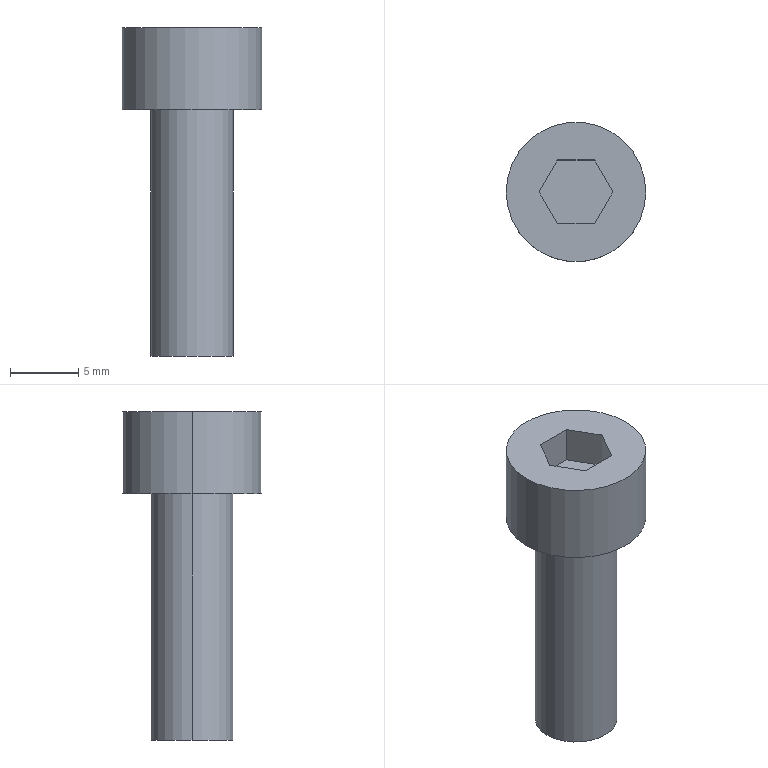Part | SolidWorks | features BaseBody 1 | 1 solid | 14 faces | box 10.2 x 10.2 x 24 mm | volume 948.077 mm3 | plane 10 | cylinder 4 | commonest cylinder face diameters 6 x2 10.2 x2
STEP:
#1=CARTESIAN_POINT('',(3.,0.,-18.));
#2=VERTEX_POINT('',#1);
#3=CARTESIAN_POINT('',(-3.,0.,-18.));
#4=VERTEX_POINT('',#3);
#5=CARTESIAN_POINT('',(0.,0.,-18.));
#6=DIRECTION('',(0.,0.,1.));
#7=DIRECTION('',(1.,0.,0.));
#8=AXIS2_PLACEMENT_3D('',#5,#6,#7);
#9=CIRCLE('',#8,3.);
#10=EDGE_CURVE('',#2,#4,#9,.T.);
#11=ORIENTED_EDGE('',*,*,#10,.T.);
#12=CARTESIAN_POINT('',(-3.,0.,0.));
#13=VERTEX_POINT('',#12);
#14=CARTESIAN_POINT('',(-3.,0.,-18.));
#15=DIRECTION('',(0.,0.,1.));
#16=VECTOR('',#15,1000.);
#17=LINE('',#14,#16);
#18=EDGE_CURVE('',#4,#13,#17,.T.);
#19=ORIENTED_EDGE('',*,*,#18,.T.);
#20=CARTESIAN_POINT('',(3.,0.,0.));
#21=VERTEX_POINT('',#20);
#22=CARTESIAN_POINT('',(0.,0.,0.));
#23=DIRECTION('',(0.,0.,-1.));
#24=DIRECTION('',(1.,0.,0.));
#25=AXIS2_PLACEMENT_3D('',#22,#23,#24);
#26=CIRCLE('',#25,3.);
#27=EDGE_CURVE('',#13,#21,#26,.T.);
#28=ORIENTED_EDGE('',*,*,#27,.T.);
#29=CARTESIAN_POINT('',(3.,0.,-18.));
#30=DIRECTION('',(0.,0.,1.));
#31=VECTOR('',#30,1000.);
#32=LINE('',#29,#31);
#33=EDGE_CURVE('',#2,#21,#32,.T.);
#34=ORIENTED_EDGE('',*,*,#33,.F.);
#35=EDGE_LOOP('',(#11,#19,#28,#34));
#36=FACE_OUTER_BOUND('',#35,.T.);
#37=CARTESIAN_POINT('',(0.,0.,-18.));
#38=DIRECTION('',(0.,0.,1.));
#39=DIRECTION('',(1.,0.,0.));
#40=AXIS2_PLACEMENT_3D('',#37,#38,#39);
#41=CYLINDRICAL_SURFACE('',#40,3.);
#42=ADVANCED_FACE('',(#36),#41,.T.);
#43=CARTESIAN_POINT('',(5.1,0.,0.));
#44=VERTEX_POINT('',#43);
#45=CARTESIAN_POINT('',(-5.1,0.,0.));
#46=VERTEX_POINT('',#45);
#47=CARTESIAN_POINT('',(0.,0.,0.));
#48=DIRECTION('',(0.,0.,1.));
#49=DIRECTION('',(1.,0.,0.));
#50=AXIS2_PLACEMENT_3D('',#47,#48,#49);
#51=CIRCLE('',#50,5.1);
#52=EDGE_CURVE('',#44,#46,#51,.T.);
#53=ORIENTED_EDGE('',*,*,#52,.T.);
#54=CARTESIAN_POINT('',(-5.1,0.,6.));
#55=VERTEX_POINT('',#54);
#56=CARTESIAN_POINT('',(-5.1,0.,0.));
#57=DIRECTION('',(0.,0.,1.));
#58=VECTOR('',#57,1000.);
#59=LINE('',#56,#58);
#60=EDGE_CURVE('',#46,#55,#59,.T.);
#61=ORIENTED_EDGE('',*,*,#60,.T.);
#62=CARTESIAN_POINT('',(5.1,0.,6.));
#63=VERTEX_POINT('',#62);
#64=CARTESIAN_POINT('',(0.,0.,6.));
#65=DIRECTION('',(0.,0.,-1.));
#66=DIRECTION('',(1.,0.,0.));
#67=AXIS2_PLACEMENT_3D('',#64,#65,#66);
#68=CIRCLE('',#67,5.1);
#69=EDGE_CURVE('',#55,#63,#68,.T.);
#70=ORIENTED_EDGE('',*,*,#69,.T.);
#71=CARTESIAN_POINT('',(5.1,0.,0.));
#72=DIRECTION('',(0.,0.,1.));
#73=VECTOR('',#72,1000.);
#74=LINE('',#71,#73);
#75=EDGE_CURVE('',#44,#63,#74,.T.);
#76=ORIENTED_EDGE('',*,*,#75,.F.);
#77=EDGE_LOOP('',(#53,#61,#70,#76));
#78=FACE_OUTER_BOUND('',#77,.T.);
#79=CARTESIAN_POINT('',(0.,0.,0.));
#80=DIRECTION('',(0.,0.,1.));
#81=DIRECTION('',(1.,0.,0.));
#82=AXIS2_PLACEMENT_3D('',#79,#80,#81);
#83=CYLINDRICAL_SURFACE('',#82,5.1);
#84=ADVANCED_FACE('',(#78),#83,.T.);
#85=ORIENTED_EDGE('',*,*,#18,.F.);
#86=CARTESIAN_POINT('',(0.,0.,-18.));
#87=DIRECTION('',(0.,0.,1.));
#88=DIRECTION('',(1.,0.,0.));
#89=AXIS2_PLACEMENT_3D('',#86,#87,#88);
#90=CIRCLE('',#89,3.);
#91=EDGE_CURVE('',#4,#2,#90,.T.);
#92=ORIENTED_EDGE('',*,*,#91,.T.);
#93=ORIENTED_EDGE('',*,*,#33,.T.);
#94=CARTESIAN_POINT('',(0.,0.,0.));
#95=DIRECTION('',(0.,0.,-1.));
#96=DIRECTION('',(1.,0.,0.));
#97=AXIS2_PLACEMENT_3D('',#94,#95,#96);
#98=CIRCLE('',#97,3.);
#99=EDGE_CURVE('',#21,#13,#98,.T.);
#100=ORIENTED_EDGE('',*,*,#99,.T.);
#101=EDGE_LOOP('',(#85,#92,#93,#100));
#102=FACE_OUTER_BOUND('',#101,.T.);
#103=CARTESIAN_POINT('',(0.,0.,-18.));
#104=DIRECTION('',(0.,0.,1.));
#105=DIRECTION('',(1.,0.,0.));
#106=AXIS2_PLACEMENT_3D('',#103,#104,#105);
#107=CYLINDRICAL_SURFACE('',#106,3.);
#108=ADVANCED_FACE('',(#102),#107,.T.);
#109=ORIENTED_EDGE('',*,*,#10,.F.);
#110=ORIENTED_EDGE('',*,*,#91,.F.);
#111=EDGE_LOOP('',(#109,#110));
#112=FACE_OUTER_BOUND('',#111,.T.);
#113=CARTESIAN_POINT('',(0.,0.,-18.));
#114=DIRECTION('',(0.,0.,1.));
#115=DIRECTION('',(1.,0.,0.));
#116=AXIS2_PLACEMENT_3D('',#113,#114,#115);
#117=PLANE('',#116);
#118=ADVANCED_FACE('',(#112),#117,.F.);
#119=ORIENTED_EDGE('',*,*,#99,.F.);
#120=ORIENTED_EDGE('',*,*,#27,.F.);
#121=EDGE_LOOP('',(#119,#120));
#122=FACE_BOUND('',#121,.T.);
#123=ORIENTED_EDGE('',*,*,#52,.F.);
#124=CARTESIAN_POINT('',(0.,0.,0.));
#125=DIRECTION('',(0.,0.,1.));
#126=DIRECTION('',(1.,0.,0.));
#127=AXIS2_PLACEMENT_3D('',#124,#125,#126);
#128=CIRCLE('',#127,5.1);
#129=EDGE_CURVE('',#46,#44,#128,.T.);
#130=ORIENTED_EDGE('',*,*,#129,.F.);
#131=EDGE_LOOP('',(#123,#130));
#132=FACE_OUTER_BOUND('',#131,.T.);
#133=CARTESIAN_POINT('',(0.,0.,0.));
#134=DIRECTION('',(0.,0.,1.));
#135=DIRECTION('',(1.,0.,0.));
#136=AXIS2_PLACEMENT_3D('',#133,#134,#135);
#137=PLANE('',#136);
#138=ADVANCED_FACE('',(#122,#132),#137,.F.);
#139=ORIENTED_EDGE('',*,*,#60,.F.);
#140=ORIENTED_EDGE('',*,*,#129,.T.);
#141=ORIENTED_EDGE('',*,*,#75,.T.);
#142=CARTESIAN_POINT('',(0.,0.,6.));
#143=DIRECTION('',(0.,0.,-1.));
#144=DIRECTION('',(1.,0.,0.));
#145=AXIS2_PLACEMENT_3D('',#142,#143,#144);
#146=CIRCLE('',#145,5.1);
#147=EDGE_CURVE('',#63,#55,#146,.T.);
#148=ORIENTED_EDGE('',*,*,#147,.T.);
#149=EDGE_LOOP('',(#139,#140,#141,#148));
#150=FACE_OUTER_BOUND('',#149,.T.);
#151=CARTESIAN_POINT('',(0.,0.,0.));
#152=DIRECTION('',(0.,0.,1.));
#153=DIRECTION('',(1.,0.,0.));
#154=AXIS2_PLACEMENT_3D('',#151,#152,#153);
#155=CYLINDRICAL_SURFACE('',#154,5.1);
#156=ADVANCED_FACE('',(#150),#155,.T.);
#157=CARTESIAN_POINT('',(-1.35,-2.338,6.));
#158=VERTEX_POINT('',#157);
#159=CARTESIAN_POINT('',(-2.7,0.,6.));
#160=VERTEX_POINT('',#159);
#161=CARTESIAN_POINT('',(-1.35,-2.338,6.));
#162=DIRECTION('',(-0.5,0.866,0.));
#163=VECTOR('',#162,1000.);
#164=LINE('',#161,#163);
#165=EDGE_CURVE('',#158,#160,#164,.T.);
#166=ORIENTED_EDGE('',*,*,#165,.T.);
#167=CARTESIAN_POINT('',(-1.35,2.338,6.));
#168=VERTEX_POINT('',#167);
#169=CARTESIAN_POINT('',(-2.7,0.,6.));
#170=DIRECTION('',(0.5,0.866,0.));
#171=VECTOR('',#170,1000.);
#172=LINE('',#169,#171);
#173=EDGE_CURVE('',#160,#168,#172,.T.);
#174=ORIENTED_EDGE('',*,*,#173,.T.);
#175=CARTESIAN_POINT('',(1.35,2.338,6.));
#176=VERTEX_POINT('',#175);
#177=CARTESIAN_POINT('',(0.,2.338,6.));
#178=DIRECTION('',(1.,0.,0.));
#179=VECTOR('',#178,1000.);
#180=LINE('',#177,#179);
#181=EDGE_CURVE('',#168,#176,#180,.T.);
#182=ORIENTED_EDGE('',*,*,#181,.T.);
#183=CARTESIAN_POINT('',(2.7,0.,6.));
#184=VERTEX_POINT('',#183);
#185=CARTESIAN_POINT('',(1.35,2.338,6.));
#186=DIRECTION('',(0.5,-0.866,0.));
#187=VECTOR('',#186,1000.);
#188=LINE('',#185,#187);
#189=EDGE_CURVE('',#176,#184,#188,.T.);
#190=ORIENTED_EDGE('',*,*,#189,.T.);
#191=CARTESIAN_POINT('',(1.35,-2.338,6.));
#192=VERTEX_POINT('',#191);
#193=CARTESIAN_POINT('',(2.7,0.,6.));
#194=DIRECTION('',(-0.5,-0.866,0.));
#195=VECTOR('',#194,1000.);
#196=LINE('',#193,#195);
#197=EDGE_CURVE('',#184,#192,#196,.T.);
#198=ORIENTED_EDGE('',*,*,#197,.T.);
#199=CARTESIAN_POINT('',(0.,-2.338,6.));
#200=DIRECTION('',(-1.,0.,0.));
#201=VECTOR('',#200,1000.);
#202=LINE('',#199,#201);
#203=EDGE_CURVE('',#192,#158,#202,.T.);
#204=ORIENTED_EDGE('',*,*,#203,.T.);
#205=EDGE_LOOP('',(#166,#174,#182,#190,#198,#204));
#206=FACE_BOUND('',#205,.T.);
#207=ORIENTED_EDGE('',*,*,#147,.F.);
#208=ORIENTED_EDGE('',*,*,#69,.F.);
#209=EDGE_LOOP('',(#207,#208));
#210=FACE_OUTER_BOUND('',#209,.T.);
#211=CARTESIAN_POINT('',(0.,0.,6.));
#212=DIRECTION('',(0.,0.,1.));
#213=DIRECTION('',(1.,0.,0.));
#214=AXIS2_PLACEMENT_3D('',#211,#212,#213);
#215=PLANE('',#214);
#216=ADVANCED_FACE('',(#206,#210),#215,.T.);
#217=ORIENTED_EDGE('',*,*,#173,.F.);
#218=CARTESIAN_POINT('',(-2.7,0.,3.3));
#219=VERTEX_POINT('',#218);
#220=CARTESIAN_POINT('',(-2.7,0.,3.3));
#221=DIRECTION('',(0.,0.,-1.));
#222=VECTOR('',#221,1000.);
#223=LINE('',#220,#222);
#224=EDGE_CURVE('',#160,#219,#223,.T.);
#225=ORIENTED_EDGE('',*,*,#224,.T.);
#226=CARTESIAN_POINT('',(-1.35,2.338,3.3));
#227=VERTEX_POINT('',#226);
#228=CARTESIAN_POINT('',(-1.35,2.338,3.3));
#229=DIRECTION('',(0.5,0.866,0.));
#230=VECTOR('',#229,1000.);
#231=LINE('',#228,#230);
#232=EDGE_CURVE('',#219,#227,#231,.T.);
#233=ORIENTED_EDGE('',*,*,#232,.T.);
#234=CARTESIAN_POINT('',(-1.35,2.338,3.3));
#235=DIRECTION('',(0.,0.,1.));
#236=VECTOR('',#235,1000.);
#237=LINE('',#234,#236);
#238=EDGE_CURVE('',#227,#168,#237,.T.);
#239=ORIENTED_EDGE('',*,*,#238,.T.);
#240=EDGE_LOOP('',(#217,#225,#233,#239));
#241=FACE_OUTER_BOUND('',#240,.T.);
#242=CARTESIAN_POINT('',(-1.35,2.338,3.3));
#243=DIRECTION('',(0.866,-0.5,0.));
#244=DIRECTION('',(0.5,0.866,0.));
#245=AXIS2_PLACEMENT_3D('',#242,#243,#244);
#246=PLANE('',#245);
#247=ADVANCED_FACE('',(#241),#246,.T.);
#248=ORIENTED_EDGE('',*,*,#165,.F.);
#249=CARTESIAN_POINT('',(-1.35,-2.338,3.3));
#250=VERTEX_POINT('',#249);
#251=CARTESIAN_POINT('',(-1.35,-2.338,3.3));
#252=DIRECTION('',(0.,0.,-1.));
#253=VECTOR('',#252,1000.);
#254=LINE('',#251,#253);
#255=EDGE_CURVE('',#158,#250,#254,.T.);
#256=ORIENTED_EDGE('',*,*,#255,.T.);
#257=CARTESIAN_POINT('',(-2.7,0.,3.3));
#258=DIRECTION('',(-0.5,0.866,0.));
#259=VECTOR('',#258,1000.);
#260=LINE('',#257,#259);
#261=EDGE_CURVE('',#250,#219,#260,.T.);
#262=ORIENTED_EDGE('',*,*,#261,.T.);
#263=ORIENTED_EDGE('',*,*,#224,.F.);
#264=EDGE_LOOP('',(#248,#256,#262,#263));
#265=FACE_OUTER_BOUND('',#264,.T.);
#266=CARTESIAN_POINT('',(-2.7,0.,3.3));
#267=DIRECTION('',(0.866,0.5,0.));
#268=DIRECTION('',(-0.5,0.866,0.));
#269=AXIS2_PLACEMENT_3D('',#266,#267,#268);
#270=PLANE('',#269);
#271=ADVANCED_FACE('',(#265),#270,.T.);
#272=ORIENTED_EDGE('',*,*,#203,.F.);
#273=CARTESIAN_POINT('',(1.35,-2.338,3.3));
#274=VERTEX_POINT('',#273);
#275=CARTESIAN_POINT('',(1.35,-2.338,3.3));
#276=DIRECTION('',(0.,0.,-1.));
#277=VECTOR('',#276,1000.);
#278=LINE('',#275,#277);
#279=EDGE_CURVE('',#192,#274,#278,.T.);
#280=ORIENTED_EDGE('',*,*,#279,.T.);
#281=CARTESIAN_POINT('',(-1.35,-2.338,3.3));
#282=DIRECTION('',(-1.,0.,0.));
#283=VECTOR('',#282,1000.);
#284=LINE('',#281,#283);
#285=EDGE_CURVE('',#274,#250,#284,.T.);
#286=ORIENTED_EDGE('',*,*,#285,.T.);
#287=ORIENTED_EDGE('',*,*,#255,.F.);
#288=EDGE_LOOP('',(#272,#280,#286,#287));
#289=FACE_OUTER_BOUND('',#288,.T.);
#290=CARTESIAN_POINT('',(-1.35,-2.338,3.3));
#291=DIRECTION('',(0.,1.,0.));
#292=DIRECTION('',(-1.,0.,0.));
#293=AXIS2_PLACEMENT_3D('',#290,#291,#292);
#294=PLANE('',#293);
#295=ADVANCED_FACE('',(#289),#294,.T.);
#296=ORIENTED_EDGE('',*,*,#197,.F.);
#297=CARTESIAN_POINT('',(2.7,0.,3.3));
#298=VERTEX_POINT('',#297);
#299=CARTESIAN_POINT('',(2.7,0.,3.3));
#300=DIRECTION('',(0.,0.,-1.));
#301=VECTOR('',#300,1000.);
#302=LINE('',#299,#301);
#303=EDGE_CURVE('',#184,#298,#302,.T.);
#304=ORIENTED_EDGE('',*,*,#303,.T.);
#305=CARTESIAN_POINT('',(1.35,-2.338,3.3));
#306=DIRECTION('',(-0.5,-0.866,0.));
#307=VECTOR('',#306,1000.);
#308=LINE('',#305,#307);
#309=EDGE_CURVE('',#298,#274,#308,.T.);
#310=ORIENTED_EDGE('',*,*,#309,.T.);
#311=ORIENTED_EDGE('',*,*,#279,.F.);
#312=EDGE_LOOP('',(#296,#304,#310,#311));
#313=FACE_OUTER_BOUND('',#312,.T.);
#314=CARTESIAN_POINT('',(1.35,-2.338,3.3));
#315=DIRECTION('',(-0.866,0.5,0.));
#316=DIRECTION('',(-0.5,-0.866,0.));
#317=AXIS2_PLACEMENT_3D('',#314,#315,#316);
#318=PLANE('',#317);
#319=ADVANCED_FACE('',(#313),#318,.T.);
#320=ORIENTED_EDGE('',*,*,#189,.F.);
#321=CARTESIAN_POINT('',(1.35,2.338,3.3));
#322=VERTEX_POINT('',#321);
#323=CARTESIAN_POINT('',(1.35,2.338,3.3));
#324=DIRECTION('',(0.,0.,-1.));
#325=VECTOR('',#324,1000.);
#326=LINE('',#323,#325);
#327=EDGE_CURVE('',#176,#322,#326,.T.);
#328=ORIENTED_EDGE('',*,*,#327,.T.);
#329=CARTESIAN_POINT('',(2.7,0.,3.3));
#330=DIRECTION('',(0.5,-0.866,0.));
#331=VECTOR('',#330,1000.);
#332=LINE('',#329,#331);
#333=EDGE_CURVE('',#322,#298,#332,.T.);
#334=ORIENTED_EDGE('',*,*,#333,.T.);
#335=ORIENTED_EDGE('',*,*,#303,.F.);
#336=EDGE_LOOP('',(#320,#328,#334,#335));
#337=FACE_OUTER_BOUND('',#336,.T.);
#338=CARTESIAN_POINT('',(2.7,0.,3.3));
#339=DIRECTION('',(-0.866,-0.5,0.));
#340=DIRECTION('',(0.5,-0.866,0.));
#341=AXIS2_PLACEMENT_3D('',#338,#339,#340);
#342=PLANE('',#341);
#343=ADVANCED_FACE('',(#337),#342,.T.);
#344=ORIENTED_EDGE('',*,*,#181,.F.);
#345=ORIENTED_EDGE('',*,*,#238,.F.);
#346=CARTESIAN_POINT('',(1.35,2.338,3.3));
#347=DIRECTION('',(1.,0.,0.));
#348=VECTOR('',#347,1000.);
#349=LINE('',#346,#348);
#350=EDGE_CURVE('',#227,#322,#349,.T.);
#351=ORIENTED_EDGE('',*,*,#350,.T.);
#352=ORIENTED_EDGE('',*,*,#327,.F.);
#353=EDGE_LOOP('',(#344,#345,#351,#352));
#354=FACE_OUTER_BOUND('',#353,.T.);
#355=CARTESIAN_POINT('',(1.35,2.338,3.3));
#356=DIRECTION('',(0.,-1.,0.));
#357=DIRECTION('',(0.,0.,-1.));
#358=AXIS2_PLACEMENT_3D('',#355,#356,#357);
#359=PLANE('',#358);
#360=ADVANCED_FACE('',(#354),#359,.T.);
#361=ORIENTED_EDGE('',*,*,#285,.F.);
#362=ORIENTED_EDGE('',*,*,#309,.F.);
#363=ORIENTED_EDGE('',*,*,#333,.F.);
#364=ORIENTED_EDGE('',*,*,#350,.F.);
#365=ORIENTED_EDGE('',*,*,#232,.F.);
#366=ORIENTED_EDGE('',*,*,#261,.F.);
#367=EDGE_LOOP('',(#361,#362,#363,#364,#365,#366));
#368=FACE_OUTER_BOUND('',#367,.T.);
#369=CARTESIAN_POINT('',(0.,0.,3.3));
#370=DIRECTION('',(0.,0.,1.));
#371=DIRECTION('',(1.,0.,0.));
#372=AXIS2_PLACEMENT_3D('',#369,#370,#371);
#373=PLANE('',#372);
#374=ADVANCED_FACE('',(#368),#373,.T.);
#375=CLOSED_SHELL('',(#42,#84,#108,#118,#138,#156,#216,#247,#271,#295,#319,#343,#360,#374));
#376=MANIFOLD_SOLID_BREP('',#375);
#377=CARTESIAN_POINT('',(0.,0.,0.));
#378=DIRECTION('',(0.,0.,1.));
#379=DIRECTION('',(1.,0.,0.));
#380=AXIS2_PLACEMENT_3D('',#377,#378,#379);
#381=(LENGTH_UNIT()NAMED_UNIT(*)SI_UNIT(.MILLI.,.METRE.));
#382=UNCERTAINTY_MEASURE_WITH_UNIT(LENGTH_MEASURE(0.00001),#381,'','');
#383=(NAMED_UNIT(*)PLANE_ANGLE_UNIT()SI_UNIT($,.RADIAN.));
#384=(NAMED_UNIT(*)SI_UNIT($,.STERADIAN.)SOLID_ANGLE_UNIT());
#385=(GEOMETRIC_REPRESENTATION_CONTEXT(3)GLOBAL_UNCERTAINTY_ASSIGNED_CONTEXT((#382))GLOBAL_UNIT_ASSIGNED_CONTEXT((#381,#383,#384))REPRESENTATION_CONTEXT('',''));
#386=ADVANCED_BREP_SHAPE_REPRESENTATION('',(#376,#380),#385);